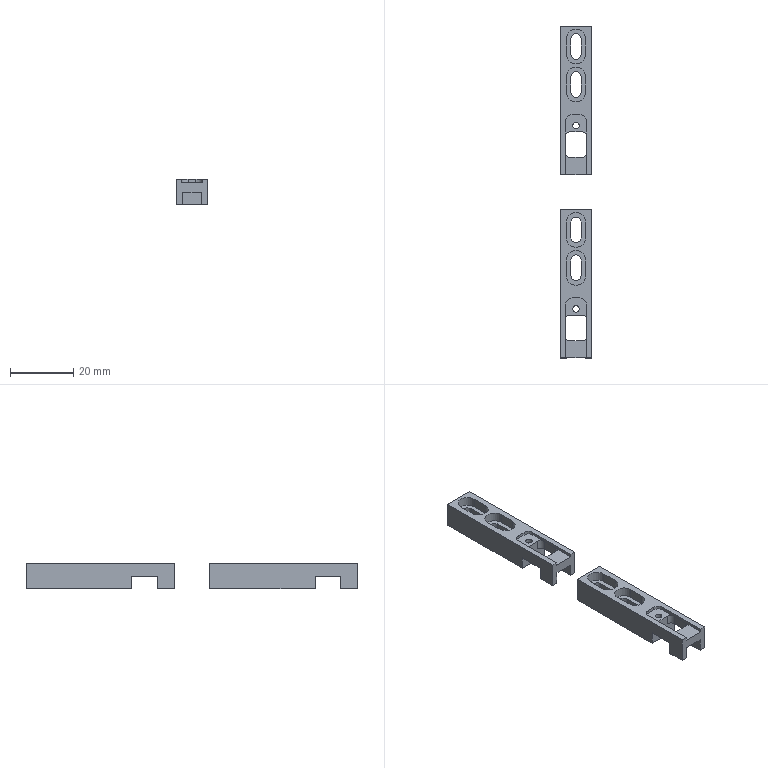CAM job | NX | 3-axis milling, drilling | part box 10 x 105 x 8 mm | stock box 15 x 110 x 10 mm
Tools:
number,name,description,diameter,corner_radius,flute_length,length,flutes
4,D4,平底铣刀-粗,4.0,0.0,25.0,75.0,2
9,D10,平底铣刀-粗,10.0,0.0,35.0,75.0,2
18,D2-J,平底铣刀-精,2.0,0.0,50.0,75.0,2
11,D3-J,平底铣刀-精,3.0,0.0,50.0,75.0,2
11,D4-J,平底铣刀-精,4.0,0.0,50.0,75.0,2
7,D6-J,平底铣刀-精,6.0,0.0,25.0,75.0,2
10,D10-J,平底铣刀-精,10.0,0.0,35.0,75.0,2
1,D80R0.8_FACEMILL,圆鼻刀-粗,80.0,0.8,50.0,75.0,2
2,D6_CHAMFERMILL,倒角刀,6.0,0.0,3.0,25.0,2
19,M2.5X0.45,丝锥,2.05,0.0,35.0,50.0,2
17,ZT2.1,钻头,2.1,0.0,35.0,50.0,2
Operations:
program,operation,operation_type,tool,method,geometry_group,spindle_rpm,surface_speed,feed_per_tooth,feed_cut,feed_plunge,cut_length_mm,path_length_mm,cut_time_min,machine_time_min
B,AUTOFACEMILL-ROUGH_COPY,FaceMilling,D10,LAYER-ROUGH-DEPTHK-STEPG,W-B,8000.0,251.327,0.1875,3000.0,100.0,1055.233,1179.883,0.3517,0.3642
B,AUTOFACEMILL-FINISH_COPY,FaceMilling,D10-J,SIDE-FINISH-DEPTHK-STEPG,W-B,8000.0,251.327,0.0625,1000.0,100.0,264.667,360.667,0.2647,0.2743
B,FLOORWALL-SPIRAL-ROUGH-S_COPY,VolumeBased25DMillingOperation,D4,LAYER-ROUGH-DEPTHK-STEPG,W-B,8000.0,100.528,0.125,2000.0,100.0,754.868,1230.564,0.3774,0.425
B,FLOORWALL-LAYER-ROUGH-M_COPY,VolumeBased25DMillingOperation,D4,LAYER-ROUGH-DEPTHK-STEPG,W-B,8000.0,100.528,0.125,2000.0,100.0,295.8,406.724,0.1479,0.159
B,FLOORWALL-SPIRAL-FINISH-S_COPY,VolumeBased25DMillingOperation,D4-J,SPIRAL-FINISH-DEPTHK-STEPG,W-B,8000.0,100.528,0.05,800.0,100.0,240.479,700.062,0.3006,0.3466
B,DRILL-CHAMFER_2,Operation,D6_CHAMFERMILL,METHOD,W-B,8000.0,150.796,0.0625,1000.0,0.0,8.65,180.377,0.0086,0.0258
B,PLANARDEBURR6X45L_COPY,SurfaceContour,D6_CHAMFERMILL,WALL_CHAMFER-DEPTH0-STEPG,W-B,6500.0,122.519,0.1154,1500.0,100.0,498.631,960.083,0.3324,0.3786
B,FLOORWALL-FINISH-SIDE-M-SELFLOOR_COPY,VolumeBased25DMillingOperation,D4-J,SIDE-FINISH-DEPTHK-STEPG,W-B,8000.0,100.528,0.05,800.0,100.0,90.826,178.428,0.1135,0.1223
A,TOPFACE,FaceMilling,D80R0.8_FACEMILL,SIDE-FINISH-DEPTHK-STEPG,W-A,4500.0,1385.0,0.1667,1500.0,100.0,199.0,295.0,0.1327,0.1423
A,FLOORWALL-SPIRAL-ROUGH-M_COPY_1,VolumeBased25DMillingOperation,D10,LAYER-ROUGH-DEPTHK-STEPG,W-A,8000.0,251.32,0.25,4000.0,100.0,4422.373,4736.571,1.106,1.137
A,SPOTDRILL-DEPTH0.8,Operation,D6_CHAMFERMILL,NONE,W-A,8000.0,150.796,0.0312,500.0,90.0,3.6,166.209,0.0072,0.0235
A,THRUHOLE-M2.5TAPDRILL,Operation,ZT2.1,NONE,W-A,3000.0,19.321,0.0333,200.0,90.0,26.0,211.009,0.13,0.1485
A,FLOORWALL-SPIRAL-ROUGH-M_COPY,VolumeBased25DMillingOperation,D4,LAYER-ROUGH-DEPTHK-STEPG,W-A,8000.0,100.528,0.125,2000.0,100.0,701.165,971.711,0.3506,0.3776
A,FLOORWALL-ROUGH_1,VolumeBased25DMillingOperation,D4,METHOD,W-A,8000.0,75.398,0.1875,3000.0,100.0,2556.2,5927.262,0.8521,1.189
A,SLOTROUGH_1,VolumeBased25DMillingOperation,D2-J,METHOD,W-A,12000.0,75.398,0.025,600.0,100.0,4001.117,4510.617,6.668,6.72
A,SLOTFINISH_1,VolumeBased25DMillingOperation,D2-J,METHOD,W-A,6000.0,113.0,0.0167,200.0,100.0,255.972,844.872,1.28,1.339
A,FLOORWALL-SPIRAL-FINISH-M_COPY,VolumeBased25DMillingOperation,D3-J,SPIRAL-FINISH-DEPTHK-STEPG,W-A,8000.0,75.396,0.0375,600.0,100.0,562.459,831.911,0.9374,0.9644
A,FLOOR-FINISH_1,VolumeBased25DMillingOperation,D3-J,METHOD,W-A,8000.0,75.398,0.0625,1000.0,100.0,162.7,906.07,0.1627,0.237
A,FLOORSIDE-FINISH_3,VolumeBased25DMillingOperation,D3-J,METHOD,W-A,8000.0,75.398,0.0625,1000.0,100.0,103.85,592.61,0.1038,0.1527
A,SELECTBODYONLY,SurfaceContour,D6_CHAMFERMILL,METHOD,W-A,8000.0,150.796,0.1875,3000.0,100.0,427.522,1268.813,0.1425,0.2266
A,DRILL-CHAMFER_1,Operation,D6_CHAMFERMILL,METHOD,W-A,8000.0,150.796,0.0312,500.0,0.0,8.95,178.977,0.0179,0.0349
A,THRUHOLE-TAPM2.5,Operation,M2.5X0.45,METHOD,W-A,1000.0,6.44,0.0002,0.45,90.0,22.0,203.009,48.889,48.907
A,FLOORWALL-FINISH-SIDE-M_COPY,VolumeBased25DMillingOperation,D6-J,SIDE-FINISH-DEPTHK-STEPG,W-A,8000.0,150.792,0.0625,1000.0,100.0,289.255,404.955,0.2893,0.3008